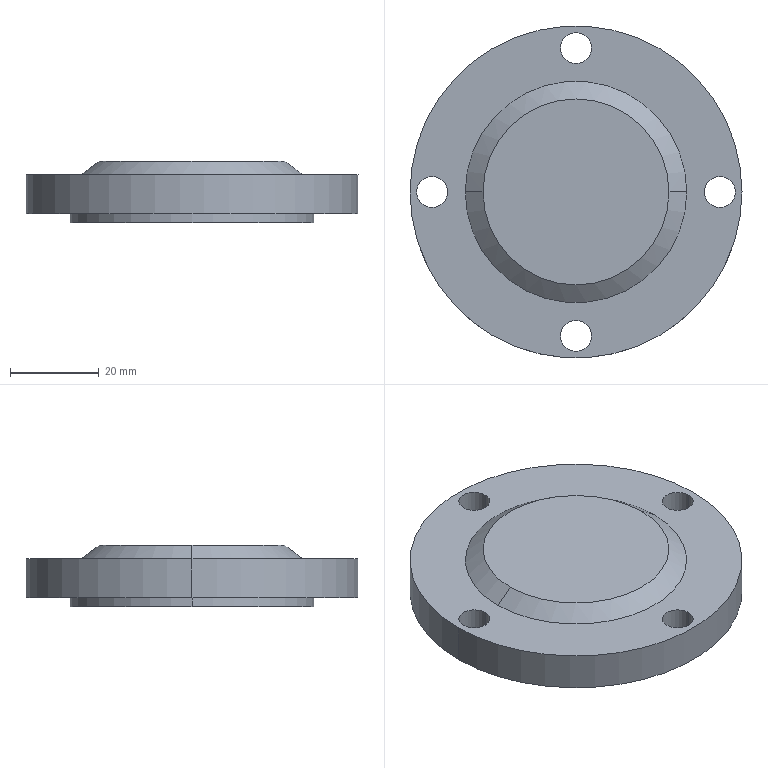Part | SolidWorks | features BaseBody 1, Chamfer 1 | 1 solid | 23 faces | box 75 x 75 x 13.8 mm | volume 30557 mm3 | cylinder 14 | plane 5 | cone 4 | commonest cylinder face diameters 7 x8 47 x2 55 x2 75 x2
STEP:
#1=CARTESIAN_POINT('',(0.,-21.5,3.4));
#2=VERTEX_POINT('',#1);
#3=CARTESIAN_POINT('',(0.,21.5,3.4));
#4=VERTEX_POINT('',#3);
#5=CARTESIAN_POINT('',(0.,0.,3.4));
#6=DIRECTION('',(0.,0.,-1.));
#7=DIRECTION('',(0.,1.,0.));
#8=AXIS2_PLACEMENT_3D('',#5,#6,#7);
#9=CIRCLE('',#8,21.5);
#10=EDGE_CURVE('',#2,#4,#9,.T.);
#11=ORIENTED_EDGE('',*,*,#10,.F.);
#12=CARTESIAN_POINT('',(0.,-23.5,1.4));
#13=VERTEX_POINT('',#12);
#14=CARTESIAN_POINT('',(0.,-21.5,3.4));
#15=DIRECTION('',(0.,-0.7071,-0.7071));
#16=VECTOR('',#15,1000.);
#17=LINE('',#14,#16);
#18=EDGE_CURVE('',#2,#13,#17,.T.);
#19=ORIENTED_EDGE('',*,*,#18,.T.);
#20=CARTESIAN_POINT('',(-23.5,0.,1.4));
#21=VERTEX_POINT('',#20);
#22=CARTESIAN_POINT('',(0.,0.,1.4));
#23=DIRECTION('',(0.,0.,1.));
#24=DIRECTION('',(0.,1.,0.));
#25=AXIS2_PLACEMENT_3D('',#22,#23,#24);
#26=CIRCLE('',#25,23.5);
#27=EDGE_CURVE('',#21,#13,#26,.T.);
#28=ORIENTED_EDGE('',*,*,#27,.F.);
#29=CARTESIAN_POINT('',(0.,23.5,1.4));
#30=VERTEX_POINT('',#29);
#31=CARTESIAN_POINT('',(0.,0.,1.4));
#32=DIRECTION('',(0.,0.,1.));
#33=DIRECTION('',(0.,1.,0.));
#34=AXIS2_PLACEMENT_3D('',#31,#32,#33);
#35=CIRCLE('',#34,23.5);
#36=EDGE_CURVE('',#30,#21,#35,.T.);
#37=ORIENTED_EDGE('',*,*,#36,.F.);
#38=CARTESIAN_POINT('',(0.,21.5,3.4));
#39=DIRECTION('',(0.,0.7071,-0.7071));
#40=VECTOR('',#39,1000.);
#41=LINE('',#38,#40);
#42=EDGE_CURVE('',#4,#30,#41,.T.);
#43=ORIENTED_EDGE('',*,*,#42,.F.);
#44=EDGE_LOOP('',(#11,#19,#28,#37,#43));
#45=FACE_OUTER_BOUND('',#44,.T.);
#46=CARTESIAN_POINT('',(0.,0.,3.4));
#47=DIRECTION('',(0.,0.,-1.));
#48=DIRECTION('',(0.,1.,0.));
#49=AXIS2_PLACEMENT_3D('',#46,#47,#48);
#50=CONICAL_SURFACE('',#49,21.5,0.7854);
#51=ADVANCED_FACE('',(#45),#50,.F.);
#52=CARTESIAN_POINT('',(-36.,0.,-4.4));
#53=VERTEX_POINT('',#52);
#54=CARTESIAN_POINT('',(-29.,0.,-4.4));
#55=VERTEX_POINT('',#54);
#56=CARTESIAN_POINT('',(-32.5,0.,-4.4));
#57=DIRECTION('',(0.,0.,1.));
#58=DIRECTION('',(1.,0.,0.));
#59=AXIS2_PLACEMENT_3D('',#56,#57,#58);
#60=CIRCLE('',#59,3.5);
#61=EDGE_CURVE('',#53,#55,#60,.T.);
#62=ORIENTED_EDGE('',*,*,#61,.F.);
#63=CARTESIAN_POINT('',(-36.,0.,4.4));
#64=VERTEX_POINT('',#63);
#65=CARTESIAN_POINT('',(-36.,0.,-5.6));
#66=DIRECTION('',(0.,0.,1.));
#67=VECTOR('',#66,1000.);
#68=LINE('',#65,#67);
#69=EDGE_CURVE('',#53,#64,#68,.T.);
#70=ORIENTED_EDGE('',*,*,#69,.T.);
#71=CARTESIAN_POINT('',(-29.,0.,4.4));
#72=VERTEX_POINT('',#71);
#73=CARTESIAN_POINT('',(-32.5,0.,4.4));
#74=DIRECTION('',(0.,0.,1.));
#75=DIRECTION('',(1.,0.,0.));
#76=AXIS2_PLACEMENT_3D('',#73,#74,#75);
#77=CIRCLE('',#76,3.5);
#78=EDGE_CURVE('',#64,#72,#77,.T.);
#79=ORIENTED_EDGE('',*,*,#78,.T.);
#80=CARTESIAN_POINT('',(-29.,0.,-5.6));
#81=DIRECTION('',(0.,0.,1.));
#82=VECTOR('',#81,1000.);
#83=LINE('',#80,#82);
#84=EDGE_CURVE('',#55,#72,#83,.T.);
#85=ORIENTED_EDGE('',*,*,#84,.F.);
#86=EDGE_LOOP('',(#62,#70,#79,#85));
#87=FACE_OUTER_BOUND('',#86,.T.);
#88=CARTESIAN_POINT('',(-32.5,0.,-5.6));
#89=DIRECTION('',(0.,0.,1.));
#90=DIRECTION('',(1.,0.,0.));
#91=AXIS2_PLACEMENT_3D('',#88,#89,#90);
#92=CYLINDRICAL_SURFACE('',#91,3.5);
#93=ADVANCED_FACE('',(#87),#92,.F.);
#94=CARTESIAN_POINT('',(-3.5,-32.5,-4.4));
#95=VERTEX_POINT('',#94);
#96=CARTESIAN_POINT('',(3.5,-32.5,-4.4));
#97=VERTEX_POINT('',#96);
#98=CARTESIAN_POINT('',(0.,-32.5,-4.4));
#99=DIRECTION('',(0.,0.,1.));
#100=DIRECTION('',(1.,0.,0.));
#101=AXIS2_PLACEMENT_3D('',#98,#99,#100);
#102=CIRCLE('',#101,3.5);
#103=EDGE_CURVE('',#95,#97,#102,.T.);
#104=ORIENTED_EDGE('',*,*,#103,.F.);
#105=CARTESIAN_POINT('',(-3.5,-32.5,4.4));
#106=VERTEX_POINT('',#105);
#107=CARTESIAN_POINT('',(-3.5,-32.5,-5.6));
#108=DIRECTION('',(0.,0.,1.));
#109=VECTOR('',#108,1000.);
#110=LINE('',#107,#109);
#111=EDGE_CURVE('',#95,#106,#110,.T.);
#112=ORIENTED_EDGE('',*,*,#111,.T.);
#113=CARTESIAN_POINT('',(3.5,-32.5,4.4));
#114=VERTEX_POINT('',#113);
#115=CARTESIAN_POINT('',(0.,-32.5,4.4));
#116=DIRECTION('',(0.,0.,1.));
#117=DIRECTION('',(1.,0.,0.));
#118=AXIS2_PLACEMENT_3D('',#115,#116,#117);
#119=CIRCLE('',#118,3.5);
#120=EDGE_CURVE('',#106,#114,#119,.T.);
#121=ORIENTED_EDGE('',*,*,#120,.T.);
#122=CARTESIAN_POINT('',(3.5,-32.5,-5.6));
#123=DIRECTION('',(0.,0.,1.));
#124=VECTOR('',#123,1000.);
#125=LINE('',#122,#124);
#126=EDGE_CURVE('',#97,#114,#125,.T.);
#127=ORIENTED_EDGE('',*,*,#126,.F.);
#128=EDGE_LOOP('',(#104,#112,#121,#127));
#129=FACE_OUTER_BOUND('',#128,.T.);
#130=CARTESIAN_POINT('',(0.,-32.5,-5.6));
#131=DIRECTION('',(0.,0.,1.));
#132=DIRECTION('',(1.,0.,0.));
#133=AXIS2_PLACEMENT_3D('',#130,#131,#132);
#134=CYLINDRICAL_SURFACE('',#133,3.5);
#135=ADVANCED_FACE('',(#129),#134,.F.);
#136=CARTESIAN_POINT('',(29.,0.,-4.4));
#137=VERTEX_POINT('',#136);
#138=CARTESIAN_POINT('',(36.,0.,-4.4));
#139=VERTEX_POINT('',#138);
#140=CARTESIAN_POINT('',(32.5,0.,-4.4));
#141=DIRECTION('',(0.,0.,1.));
#142=DIRECTION('',(1.,0.,0.));
#143=AXIS2_PLACEMENT_3D('',#140,#141,#142);
#144=CIRCLE('',#143,3.5);
#145=EDGE_CURVE('',#137,#139,#144,.T.);
#146=ORIENTED_EDGE('',*,*,#145,.F.);
#147=CARTESIAN_POINT('',(29.,0.,4.4));
#148=VERTEX_POINT('',#147);
#149=CARTESIAN_POINT('',(29.,0.,-5.6));
#150=DIRECTION('',(0.,0.,1.));
#151=VECTOR('',#150,1000.);
#152=LINE('',#149,#151);
#153=EDGE_CURVE('',#137,#148,#152,.T.);
#154=ORIENTED_EDGE('',*,*,#153,.T.);
#155=CARTESIAN_POINT('',(36.,0.,4.4));
#156=VERTEX_POINT('',#155);
#157=CARTESIAN_POINT('',(32.5,0.,4.4));
#158=DIRECTION('',(0.,0.,1.));
#159=DIRECTION('',(1.,0.,0.));
#160=AXIS2_PLACEMENT_3D('',#157,#158,#159);
#161=CIRCLE('',#160,3.5);
#162=EDGE_CURVE('',#148,#156,#161,.T.);
#163=ORIENTED_EDGE('',*,*,#162,.T.);
#164=CARTESIAN_POINT('',(36.,0.,-5.6));
#165=DIRECTION('',(0.,0.,1.));
#166=VECTOR('',#165,1000.);
#167=LINE('',#164,#166);
#168=EDGE_CURVE('',#139,#156,#167,.T.);
#169=ORIENTED_EDGE('',*,*,#168,.F.);
#170=EDGE_LOOP('',(#146,#154,#163,#169));
#171=FACE_OUTER_BOUND('',#170,.T.);
#172=CARTESIAN_POINT('',(32.5,0.,-5.6));
#173=DIRECTION('',(0.,0.,1.));
#174=DIRECTION('',(1.,0.,0.));
#175=AXIS2_PLACEMENT_3D('',#172,#173,#174);
#176=CYLINDRICAL_SURFACE('',#175,3.5);
#177=ADVANCED_FACE('',(#171),#176,.F.);
#178=CARTESIAN_POINT('',(-3.5,32.5,-4.4));
#179=VERTEX_POINT('',#178);
#180=CARTESIAN_POINT('',(3.5,32.5,-4.4));
#181=VERTEX_POINT('',#180);
#182=CARTESIAN_POINT('',(0.,32.5,-4.4));
#183=DIRECTION('',(0.,0.,1.));
#184=DIRECTION('',(1.,0.,0.));
#185=AXIS2_PLACEMENT_3D('',#182,#183,#184);
#186=CIRCLE('',#185,3.5);
#187=EDGE_CURVE('',#179,#181,#186,.T.);
#188=ORIENTED_EDGE('',*,*,#187,.F.);
#189=CARTESIAN_POINT('',(-3.5,32.5,4.4));
#190=VERTEX_POINT('',#189);
#191=CARTESIAN_POINT('',(-3.5,32.5,-5.6));
#192=DIRECTION('',(0.,0.,1.));
#193=VECTOR('',#192,1000.);
#194=LINE('',#191,#193);
#195=EDGE_CURVE('',#179,#190,#194,.T.);
#196=ORIENTED_EDGE('',*,*,#195,.T.);
#197=CARTESIAN_POINT('',(3.5,32.5,4.4));
#198=VERTEX_POINT('',#197);
#199=CARTESIAN_POINT('',(0.,32.5,4.4));
#200=DIRECTION('',(0.,0.,1.));
#201=DIRECTION('',(1.,0.,0.));
#202=AXIS2_PLACEMENT_3D('',#199,#200,#201);
#203=CIRCLE('',#202,3.5);
#204=EDGE_CURVE('',#190,#198,#203,.T.);
#205=ORIENTED_EDGE('',*,*,#204,.T.);
#206=CARTESIAN_POINT('',(3.5,32.5,-5.6));
#207=DIRECTION('',(0.,0.,1.));
#208=VECTOR('',#207,1000.);
#209=LINE('',#206,#208);
#210=EDGE_CURVE('',#181,#198,#209,.T.);
#211=ORIENTED_EDGE('',*,*,#210,.F.);
#212=EDGE_LOOP('',(#188,#196,#205,#211));
#213=FACE_OUTER_BOUND('',#212,.T.);
#214=CARTESIAN_POINT('',(0.,32.5,-5.6));
#215=DIRECTION('',(0.,0.,1.));
#216=DIRECTION('',(1.,0.,0.));
#217=AXIS2_PLACEMENT_3D('',#214,#215,#216);
#218=CYLINDRICAL_SURFACE('',#217,3.5);
#219=ADVANCED_FACE('',(#213),#218,.F.);
#220=ORIENTED_EDGE('',*,*,#27,.T.);
#221=CARTESIAN_POINT('',(23.5,0.,1.4));
#222=VERTEX_POINT('',#221);
#223=CARTESIAN_POINT('',(0.,0.,1.4));
#224=DIRECTION('',(0.,0.,1.));
#225=DIRECTION('',(0.,1.,0.));
#226=AXIS2_PLACEMENT_3D('',#223,#224,#225);
#227=CIRCLE('',#226,23.5);
#228=EDGE_CURVE('',#13,#222,#227,.T.);
#229=ORIENTED_EDGE('',*,*,#228,.T.);
#230=CARTESIAN_POINT('',(23.5,0.,-6.4));
#231=VERTEX_POINT('',#230);
#232=CARTESIAN_POINT('',(23.5,0.,3.4));
#233=DIRECTION('',(0.,0.,-1.));
#234=VECTOR('',#233,1000.);
#235=LINE('',#232,#234);
#236=EDGE_CURVE('',#222,#231,#235,.T.);
#237=ORIENTED_EDGE('',*,*,#236,.T.);
#238=CARTESIAN_POINT('',(-23.5,0.,-6.4));
#239=VERTEX_POINT('',#238);
#240=CARTESIAN_POINT('',(0.,0.,-6.4));
#241=DIRECTION('',(0.,0.,-1.));
#242=DIRECTION('',(-1.,0.,0.));
#243=AXIS2_PLACEMENT_3D('',#240,#241,#242);
#244=CIRCLE('',#243,23.5);
#245=EDGE_CURVE('',#231,#239,#244,.T.);
#246=ORIENTED_EDGE('',*,*,#245,.T.);
#247=CARTESIAN_POINT('',(-23.5,0.,3.4));
#248=DIRECTION('',(0.,0.,-1.));
#249=VECTOR('',#248,1000.);
#250=LINE('',#247,#249);
#251=EDGE_CURVE('',#21,#239,#250,.T.);
#252=ORIENTED_EDGE('',*,*,#251,.F.);
#253=EDGE_LOOP('',(#220,#229,#237,#246,#252));
#254=FACE_OUTER_BOUND('',#253,.T.);
#255=CARTESIAN_POINT('',(0.,0.,3.4));
#256=DIRECTION('',(0.,0.,-1.));
#257=DIRECTION('',(-1.,0.,0.));
#258=AXIS2_PLACEMENT_3D('',#255,#256,#257);
#259=CYLINDRICAL_SURFACE('',#258,23.5);
#260=ADVANCED_FACE('',(#254),#259,.F.);
#261=CARTESIAN_POINT('',(27.5,0.,-6.4));
#262=VERTEX_POINT('',#261);
#263=CARTESIAN_POINT('',(-27.5,0.,-6.4));
#264=VERTEX_POINT('',#263);
#265=CARTESIAN_POINT('',(0.,0.,-6.4));
#266=DIRECTION('',(0.,0.,1.));
#267=DIRECTION('',(1.,0.,0.));
#268=AXIS2_PLACEMENT_3D('',#265,#266,#267);
#269=CIRCLE('',#268,27.5);
#270=EDGE_CURVE('',#262,#264,#269,.T.);
#271=ORIENTED_EDGE('',*,*,#270,.T.);
#272=CARTESIAN_POINT('',(-27.5,0.,-4.4));
#273=VERTEX_POINT('',#272);
#274=CARTESIAN_POINT('',(-27.5,0.,-6.6));
#275=DIRECTION('',(0.,0.,1.));
#276=VECTOR('',#275,1000.);
#277=LINE('',#274,#276);
#278=EDGE_CURVE('',#264,#273,#277,.T.);
#279=ORIENTED_EDGE('',*,*,#278,.T.);
#280=CARTESIAN_POINT('',(27.5,0.,-4.4));
#281=VERTEX_POINT('',#280);
#282=CARTESIAN_POINT('',(0.,0.,-4.4));
#283=DIRECTION('',(0.,0.,-1.));
#284=DIRECTION('',(1.,0.,0.));
#285=AXIS2_PLACEMENT_3D('',#282,#283,#284);
#286=CIRCLE('',#285,27.5);
#287=EDGE_CURVE('',#273,#281,#286,.T.);
#288=ORIENTED_EDGE('',*,*,#287,.T.);
#289=CARTESIAN_POINT('',(27.5,0.,-6.6));
#290=DIRECTION('',(0.,0.,1.));
#291=VECTOR('',#290,1000.);
#292=LINE('',#289,#291);
#293=EDGE_CURVE('',#262,#281,#292,.T.);
#294=ORIENTED_EDGE('',*,*,#293,.F.);
#295=EDGE_LOOP('',(#271,#279,#288,#294));
#296=FACE_OUTER_BOUND('',#295,.T.);
#297=CARTESIAN_POINT('',(0.,0.,-6.6));
#298=DIRECTION('',(0.,0.,1.));
#299=DIRECTION('',(1.,0.,0.));
#300=AXIS2_PLACEMENT_3D('',#297,#298,#299);
#301=CYLINDRICAL_SURFACE('',#300,27.5);
#302=ADVANCED_FACE('',(#296),#301,.T.);
#303=CARTESIAN_POINT('',(-21.,0.,7.4));
#304=VERTEX_POINT('',#303);
#305=CARTESIAN_POINT('',(21.,0.,7.4));
#306=VERTEX_POINT('',#305);
#307=CARTESIAN_POINT('',(0.,0.,7.4));
#308=DIRECTION('',(0.,0.,-1.));
#309=DIRECTION('',(-1.,0.,0.));
#310=AXIS2_PLACEMENT_3D('',#307,#308,#309);
#311=CIRCLE('',#310,21.);
#312=EDGE_CURVE('',#304,#306,#311,.T.);
#313=ORIENTED_EDGE('',*,*,#312,.T.);
#314=CARTESIAN_POINT('',(25.,0.,4.4));
#315=VERTEX_POINT('',#314);
#316=CARTESIAN_POINT('',(21.,0.,7.4));
#317=DIRECTION('',(0.8,0.,-0.6));
#318=VECTOR('',#317,1000.);
#319=LINE('',#316,#318);
#320=EDGE_CURVE('',#306,#315,#319,.T.);
#321=ORIENTED_EDGE('',*,*,#320,.T.);
#322=CARTESIAN_POINT('',(-25.,0.,4.4));
#323=VERTEX_POINT('',#322);
#324=CARTESIAN_POINT('',(0.,0.,4.4));
#325=DIRECTION('',(0.,0.,-1.));
#326=DIRECTION('',(-1.,0.,0.));
#327=AXIS2_PLACEMENT_3D('',#324,#325,#326);
#328=CIRCLE('',#327,25.);
#329=EDGE_CURVE('',#323,#315,#328,.T.);
#330=ORIENTED_EDGE('',*,*,#329,.F.);
#331=CARTESIAN_POINT('',(-21.,0.,7.4));
#332=DIRECTION('',(-0.8,0.,-0.6));
#333=VECTOR('',#332,1000.);
#334=LINE('',#331,#333);
#335=EDGE_CURVE('',#304,#323,#334,.T.);
#336=ORIENTED_EDGE('',*,*,#335,.F.);
#337=EDGE_LOOP('',(#313,#321,#330,#336));
#338=FACE_OUTER_BOUND('',#337,.T.);
#339=CARTESIAN_POINT('',(0.,0.,7.4));
#340=DIRECTION('',(0.,0.,-1.));
#341=DIRECTION('',(-1.,0.,0.));
#342=AXIS2_PLACEMENT_3D('',#339,#340,#341);
#343=CONICAL_SURFACE('',#342,21.,0.9273);
#344=ADVANCED_FACE('',(#338),#343,.T.);
#345=CARTESIAN_POINT('',(37.5,0.,4.4));
#346=VERTEX_POINT('',#345);
#347=CARTESIAN_POINT('',(-37.5,0.,4.4));
#348=VERTEX_POINT('',#347);
#349=CARTESIAN_POINT('',(0.,0.,4.4));
#350=DIRECTION('',(0.,0.,1.));
#351=DIRECTION('',(1.,0.,0.));
#352=AXIS2_PLACEMENT_3D('',#349,#350,#351);
#353=CIRCLE('',#352,37.5);
#354=EDGE_CURVE('',#346,#348,#353,.T.);
#355=ORIENTED_EDGE('',*,*,#354,.F.);
#356=CARTESIAN_POINT('',(37.5,0.,-4.4));
#357=VERTEX_POINT('',#356);
#358=CARTESIAN_POINT('',(37.5,0.,4.4));
#359=DIRECTION('',(0.,0.,-1.));
#360=VECTOR('',#359,1000.);
#361=LINE('',#358,#360);
#362=EDGE_CURVE('',#346,#357,#361,.T.);
#363=ORIENTED_EDGE('',*,*,#362,.T.);
#364=CARTESIAN_POINT('',(-37.5,0.,-4.4));
#365=VERTEX_POINT('',#364);
#366=CARTESIAN_POINT('',(0.,0.,-4.4));
#367=DIRECTION('',(0.,0.,1.));
#368=DIRECTION('',(1.,0.,0.));
#369=AXIS2_PLACEMENT_3D('',#366,#367,#368);
#370=CIRCLE('',#369,37.5);
#371=EDGE_CURVE('',#357,#365,#370,.T.);
#372=ORIENTED_EDGE('',*,*,#371,.T.);
#373=CARTESIAN_POINT('',(-37.5,0.,4.4));
#374=DIRECTION('',(0.,0.,-1.));
#375=VECTOR('',#374,1000.);
#376=LINE('',#373,#375);
#377=EDGE_CURVE('',#348,#365,#376,.T.);
#378=ORIENTED_EDGE('',*,*,#377,.F.);
#379=EDGE_LOOP('',(#355,#363,#372,#378));
#380=FACE_OUTER_BOUND('',#379,.T.);
#381=CARTESIAN_POINT('',(0.,0.,4.4));
#382=DIRECTION('',(0.,0.,-1.));
#383=DIRECTION('',(-1.,0.,0.));
#384=AXIS2_PLACEMENT_3D('',#381,#382,#383);
#385=CYLINDRICAL_SURFACE('',#384,37.5);
#386=ADVANCED_FACE('',(#380),#385,.T.);
#387=CARTESIAN_POINT('',(0.,0.,3.4));
#388=DIRECTION('',(0.,0.,-1.));
#389=DIRECTION('',(0.,1.,0.));
#390=AXIS2_PLACEMENT_3D('',#387,#388,#389);
#391=CIRCLE('',#390,21.5);
#392=EDGE_CURVE('',#4,#2,#391,.T.);
#393=ORIENTED_EDGE('',*,*,#392,.T.);
#394=ORIENTED_EDGE('',*,*,#10,.T.);
#395=EDGE_LOOP('',(#393,#394));
#396=FACE_OUTER_BOUND('',#395,.T.);
#397=CARTESIAN_POINT('',(0.,0.,3.4));
#398=DIRECTION('',(0.,0.,-1.));
#399=DIRECTION('',(-1.,0.,0.));
#400=AXIS2_PLACEMENT_3D('',#397,#398,#399);
#401=PLANE('',#400);
#402=ADVANCED_FACE('',(#396),#401,.T.);
#403=ORIENTED_EDGE('',*,*,#312,.F.);
#404=CARTESIAN_POINT('',(0.,0.,7.4));
#405=DIRECTION('',(0.,0.,-1.));
#406=DIRECTION('',(-1.,0.,0.));
#407=AXIS2_PLACEMENT_3D('',#404,#405,#406);
#408=CIRCLE('',#407,21.);
#409=EDGE_CURVE('',#306,#304,#408,.T.);
#410=ORIENTED_EDGE('',*,*,#409,.F.);
#411=EDGE_LOOP('',(#403,#410));
#412=FACE_OUTER_BOUND('',#411,.T.);
#413=CARTESIAN_POINT('',(0.,0.,7.4));
#414=DIRECTION('',(0.,0.,-1.));
#415=DIRECTION('',(-1.,0.,0.));
#416=AXIS2_PLACEMENT_3D('',#413,#414,#415);
#417=PLANE('',#416);
#418=ADVANCED_FACE('',(#412),#417,.F.);
#419=CARTESIAN_POINT('',(0.,0.,-4.4));
#420=DIRECTION('',(0.,0.,-1.));
#421=DIRECTION('',(1.,0.,0.));
#422=AXIS2_PLACEMENT_3D('',#419,#420,#421);
#423=CIRCLE('',#422,27.5);
#424=EDGE_CURVE('',#281,#273,#423,.T.);
#425=ORIENTED_EDGE('',*,*,#424,.F.);
#426=ORIENTED_EDGE('',*,*,#287,.F.);
#427=EDGE_LOOP('',(#425,#426));
#428=FACE_BOUND('',#427,.T.);
#429=CARTESIAN_POINT('',(0.,32.5,-4.4));
#430=DIRECTION('',(0.,0.,1.));
#431=DIRECTION('',(1.,0.,0.));
#432=AXIS2_PLACEMENT_3D('',#429,#430,#431);
#433=CIRCLE('',#432,3.5);
#434=EDGE_CURVE('',#181,#179,#433,.T.);
#435=ORIENTED_EDGE('',*,*,#434,.T.);
#436=ORIENTED_EDGE('',*,*,#187,.T.);
#437=EDGE_LOOP('',(#435,#436));
#438=FACE_BOUND('',#437,.T.);
#439=CARTESIAN_POINT('',(32.5,0.,-4.4));
#440=DIRECTION('',(0.,0.,1.));
#441=DIRECTION('',(1.,0.,0.));
#442=AXIS2_PLACEMENT_3D('',#439,#440,#441);
#443=CIRCLE('',#442,3.5);
#444=EDGE_CURVE('',#139,#137,#443,.T.);
#445=ORIENTED_EDGE('',*,*,#444,.T.);
#446=ORIENTED_EDGE('',*,*,#145,.T.);
#447=EDGE_LOOP('',(#445,#446));
#448=FACE_BOUND('',#447,.T.);
#449=CARTESIAN_POINT('',(0.,-32.5,-4.4));
#450=DIRECTION('',(0.,0.,1.));
#451=DIRECTION('',(1.,0.,0.));
#452=AXIS2_PLACEMENT_3D('',#449,#450,#451);
#453=CIRCLE('',#452,3.5);
#454=EDGE_CURVE('',#97,#95,#453,.T.);
#455=ORIENTED_EDGE('',*,*,#454,.T.);
#456=ORIENTED_EDGE('',*,*,#103,.T.);
#457=EDGE_LOOP('',(#455,#456));
#458=FACE_BOUND('',#457,.T.);
#459=CARTESIAN_POINT('',(-32.5,0.,-4.4));
#460=DIRECTION('',(0.,0.,1.));
#461=DIRECTION('',(1.,0.,0.));
#462=AXIS2_PLACEMENT_3D('',#459,#460,#461);
#463=CIRCLE('',#462,3.5);
#464=EDGE_CURVE('',#55,#53,#463,.T.);
#465=ORIENTED_EDGE('',*,*,#464,.T.);
#466=ORIENTED_EDGE('',*,*,#61,.T.);
#467=EDGE_LOOP('',(#465,#466));
#468=FACE_BOUND('',#467,.T.);
#469=CARTESIAN_POINT('',(0.,0.,-4.4));
#470=DIRECTION('',(0.,0.,1.));
#471=DIRECTION('',(1.,0.,0.));
#472=AXIS2_PLACEMENT_3D('',#469,#470,#471);
#473=CIRCLE('',#472,37.5);
#474=EDGE_CURVE('',#365,#357,#473,.T.);
#475=ORIENTED_EDGE('',*,*,#474,.F.);
#476=ORIENTED_EDGE('',*,*,#371,.F.);
#477=EDGE_LOOP('',(#475,#476));
#478=FACE_OUTER_BOUND('',#477,.T.);
#479=CARTESIAN_POINT('',(0.,0.,-4.4));
#480=DIRECTION('',(0.,0.,1.));
#481=DIRECTION('',(0.,-1.,0.));
#482=AXIS2_PLACEMENT_3D('',#479,#480,#481);
#483=PLANE('',#482);
#484=ADVANCED_FACE('',(#428,#438,#448,#458,#468,#478),#483,.F.);
#485=ORIENTED_EDGE('',*,*,#329,.T.);
#486=CARTESIAN_POINT('',(0.,0.,4.4));
#487=DIRECTION('',(0.,0.,-1.));
#488=DIRECTION('',(-1.,0.,0.));
#489=AXIS2_PLACEMENT_3D('',#486,#487,#488);
#490=CIRCLE('',#489,25.);
#491=EDGE_CURVE('',#315,#323,#490,.T.);
#492=ORIENTED_EDGE('',*,*,#491,.T.);
#493=EDGE_LOOP('',(#485,#492));
#494=FACE_BOUND('',#493,.T.);
#495=CARTESIAN_POINT('',(0.,32.5,4.4));
#496=DIRECTION('',(0.,0.,1.));
#497=DIRECTION('',(1.,0.,0.));
#498=AXIS2_PLACEMENT_3D('',#495,#496,#497);
#499=CIRCLE('',#498,3.5);
#500=EDGE_CURVE('',#198,#190,#499,.T.);
#501=ORIENTED_EDGE('',*,*,#500,.F.);
#502=ORIENTED_EDGE('',*,*,#204,.F.);
#503=EDGE_LOOP('',(#501,#502));
#504=FACE_BOUND('',#503,.T.);
#505=CARTESIAN_POINT('',(32.5,0.,4.4));
#506=DIRECTION('',(0.,0.,1.));
#507=DIRECTION('',(1.,0.,0.));
#508=AXIS2_PLACEMENT_3D('',#505,#506,#507);
#509=CIRCLE('',#508,3.5);
#510=EDGE_CURVE('',#156,#148,#509,.T.);
#511=ORIENTED_EDGE('',*,*,#510,.F.);
#512=ORIENTED_EDGE('',*,*,#162,.F.);
#513=EDGE_LOOP('',(#511,#512));
#514=FACE_BOUND('',#513,.T.);
#515=CARTESIAN_POINT('',(0.,-32.5,4.4));
#516=DIRECTION('',(0.,0.,1.));
#517=DIRECTION('',(1.,0.,0.));
#518=AXIS2_PLACEMENT_3D('',#515,#516,#517);
#519=CIRCLE('',#518,3.5);
#520=EDGE_CURVE('',#114,#106,#519,.T.);
#521=ORIENTED_EDGE('',*,*,#520,.F.);
#522=ORIENTED_EDGE('',*,*,#120,.F.);
#523=EDGE_LOOP('',(#521,#522));
#524=FACE_BOUND('',#523,.T.);
#525=CARTESIAN_POINT('',(-32.5,0.,4.4));
#526=DIRECTION('',(0.,0.,1.));
#527=DIRECTION('',(1.,0.,0.));
#528=AXIS2_PLACEMENT_3D('',#525,#526,#527);
#529=CIRCLE('',#528,3.5);
#530=EDGE_CURVE('',#72,#64,#529,.T.);
#531=ORIENTED_EDGE('',*,*,#530,.F.);
#532=ORIENTED_EDGE('',*,*,#78,.F.);
#533=EDGE_LOOP('',(#531,#532));
#534=FACE_BOUND('',#533,.T.);
#535=CARTESIAN_POINT('',(0.,0.,4.4));
#536=DIRECTION('',(0.,0.,1.));
#537=DIRECTION('',(1.,0.,0.));
#538=AXIS2_PLACEMENT_3D('',#535,#536,#537);
#539=CIRCLE('',#538,37.5);
#540=EDGE_CURVE('',#348,#346,#539,.T.);
#541=ORIENTED_EDGE('',*,*,#540,.T.);
#542=ORIENTED_EDGE('',*,*,#354,.T.);
#543=EDGE_LOOP('',(#541,#542));
#544=FACE_OUTER_BOUND('',#543,.T.);
#545=CARTESIAN_POINT('',(0.,0.,4.4));
#546=DIRECTION('',(0.,0.,1.));
#547=DIRECTION('',(0.,-1.,0.));
#548=AXIS2_PLACEMENT_3D('',#545,#546,#547);
#549=PLANE('',#548);
#550=ADVANCED_FACE('',(#494,#504,#514,#524,#534,#544),#549,.T.);
#551=ORIENTED_EDGE('',*,*,#362,.F.);
#552=ORIENTED_EDGE('',*,*,#540,.F.);
#553=ORIENTED_EDGE('',*,*,#377,.T.);
#554=ORIENTED_EDGE('',*,*,#474,.T.);
#555=EDGE_LOOP('',(#551,#552,#553,#554));
#556=FACE_OUTER_BOUND('',#555,.T.);
#557=CARTESIAN_POINT('',(0.,0.,4.4));
#558=DIRECTION('',(0.,0.,-1.));
#559=DIRECTION('',(-1.,0.,0.));
#560=AXIS2_PLACEMENT_3D('',#557,#558,#559);
#561=CYLINDRICAL_SURFACE('',#560,37.5);
#562=ADVANCED_FACE('',(#556),#561,.T.);
#563=ORIENTED_EDGE('',*,*,#320,.F.);
#564=ORIENTED_EDGE('',*,*,#409,.T.);
#565=ORIENTED_EDGE('',*,*,#335,.T.);
#566=ORIENTED_EDGE('',*,*,#491,.F.);
#567=EDGE_LOOP('',(#563,#564,#565,#566));
#568=FACE_OUTER_BOUND('',#567,.T.);
#569=CARTESIAN_POINT('',(0.,0.,7.4));
#570=DIRECTION('',(0.,0.,-1.));
#571=DIRECTION('',(-1.,0.,0.));
#572=AXIS2_PLACEMENT_3D('',#569,#570,#571);
#573=CONICAL_SURFACE('',#572,21.,0.9273);
#574=ADVANCED_FACE('',(#568),#573,.T.);
#575=ORIENTED_EDGE('',*,*,#278,.F.);
#576=CARTESIAN_POINT('',(0.,0.,-6.4));
#577=DIRECTION('',(0.,0.,1.));
#578=DIRECTION('',(1.,0.,0.));
#579=AXIS2_PLACEMENT_3D('',#576,#577,#578);
#580=CIRCLE('',#579,27.5);
#581=EDGE_CURVE('',#264,#262,#580,.T.);
#582=ORIENTED_EDGE('',*,*,#581,.T.);
#583=ORIENTED_EDGE('',*,*,#293,.T.);
#584=ORIENTED_EDGE('',*,*,#424,.T.);
#585=EDGE_LOOP('',(#575,#582,#583,#584));
#586=FACE_OUTER_BOUND('',#585,.T.);
#587=CARTESIAN_POINT('',(0.,0.,-6.6));
#588=DIRECTION('',(0.,0.,1.));
#589=DIRECTION('',(1.,0.,0.));
#590=AXIS2_PLACEMENT_3D('',#587,#588,#589);
#591=CYLINDRICAL_SURFACE('',#590,27.5);
#592=ADVANCED_FACE('',(#586),#591,.T.);
#593=ORIENTED_EDGE('',*,*,#236,.F.);
#594=CARTESIAN_POINT('',(0.,0.,1.4));
#595=DIRECTION('',(0.,0.,1.));
#596=DIRECTION('',(0.,1.,0.));
#597=AXIS2_PLACEMENT_3D('',#594,#595,#596);
#598=CIRCLE('',#597,23.5);
#599=EDGE_CURVE('',#222,#30,#598,.T.);
#600=ORIENTED_EDGE('',*,*,#599,.T.);
#601=ORIENTED_EDGE('',*,*,#36,.T.);
#602=ORIENTED_EDGE('',*,*,#251,.T.);
#603=CARTESIAN_POINT('',(0.,0.,-6.4));
#604=DIRECTION('',(0.,0.,-1.));
#605=DIRECTION('',(-1.,0.,0.));
#606=AXIS2_PLACEMENT_3D('',#603,#604,#605);
#607=CIRCLE('',#606,23.5);
#608=EDGE_CURVE('',#239,#231,#607,.T.);
#609=ORIENTED_EDGE('',*,*,#608,.T.);
#610=EDGE_LOOP('',(#593,#600,#601,#602,#609));
#611=FACE_OUTER_BOUND('',#610,.T.);
#612=CARTESIAN_POINT('',(0.,0.,3.4));
#613=DIRECTION('',(0.,0.,-1.));
#614=DIRECTION('',(-1.,0.,0.));
#615=AXIS2_PLACEMENT_3D('',#612,#613,#614);
#616=CYLINDRICAL_SURFACE('',#615,23.5);
#617=ADVANCED_FACE('',(#611),#616,.F.);
#618=ORIENTED_EDGE('',*,*,#195,.F.);
#619=ORIENTED_EDGE('',*,*,#434,.F.);
#620=ORIENTED_EDGE('',*,*,#210,.T.);
#621=ORIENTED_EDGE('',*,*,#500,.T.);
#622=EDGE_LOOP('',(#618,#619,#620,#621));
#623=FACE_OUTER_BOUND('',#622,.T.);
#624=CARTESIAN_POINT('',(0.,32.5,-5.6));
#625=DIRECTION('',(0.,0.,1.));
#626=DIRECTION('',(1.,0.,0.));
#627=AXIS2_PLACEMENT_3D('',#624,#625,#626);
#628=CYLINDRICAL_SURFACE('',#627,3.5);
#629=ADVANCED_FACE('',(#623),#628,.F.);
#630=ORIENTED_EDGE('',*,*,#153,.F.);
#631=ORIENTED_EDGE('',*,*,#444,.F.);
#632=ORIENTED_EDGE('',*,*,#168,.T.);
#633=ORIENTED_EDGE('',*,*,#510,.T.);
#634=EDGE_LOOP('',(#630,#631,#632,#633));
#635=FACE_OUTER_BOUND('',#634,.T.);
#636=CARTESIAN_POINT('',(32.5,0.,-5.6));
#637=DIRECTION('',(0.,0.,1.));
#638=DIRECTION('',(1.,0.,0.));
#639=AXIS2_PLACEMENT_3D('',#636,#637,#638);
#640=CYLINDRICAL_SURFACE('',#639,3.5);
#641=ADVANCED_FACE('',(#635),#640,.F.);
#642=ORIENTED_EDGE('',*,*,#111,.F.);
#643=ORIENTED_EDGE('',*,*,#454,.F.);
#644=ORIENTED_EDGE('',*,*,#126,.T.);
#645=ORIENTED_EDGE('',*,*,#520,.T.);
#646=EDGE_LOOP('',(#642,#643,#644,#645));
#647=FACE_OUTER_BOUND('',#646,.T.);
#648=CARTESIAN_POINT('',(0.,-32.5,-5.6));
#649=DIRECTION('',(0.,0.,1.));
#650=DIRECTION('',(1.,0.,0.));
#651=AXIS2_PLACEMENT_3D('',#648,#649,#650);
#652=CYLINDRICAL_SURFACE('',#651,3.5);
#653=ADVANCED_FACE('',(#647),#652,.F.);
#654=ORIENTED_EDGE('',*,*,#69,.F.);
#655=ORIENTED_EDGE('',*,*,#464,.F.);
#656=ORIENTED_EDGE('',*,*,#84,.T.);
#657=ORIENTED_EDGE('',*,*,#530,.T.);
#658=EDGE_LOOP('',(#654,#655,#656,#657));
#659=FACE_OUTER_BOUND('',#658,.T.);
#660=CARTESIAN_POINT('',(-32.5,0.,-5.6));
#661=DIRECTION('',(0.,0.,1.));
#662=DIRECTION('',(1.,0.,0.));
#663=AXIS2_PLACEMENT_3D('',#660,#661,#662);
#664=CYLINDRICAL_SURFACE('',#663,3.5);
#665=ADVANCED_FACE('',(#659),#664,.F.);
#666=ORIENTED_EDGE('',*,*,#608,.F.);
#667=ORIENTED_EDGE('',*,*,#245,.F.);
#668=EDGE_LOOP('',(#666,#667));
#669=FACE_BOUND('',#668,.T.);
#670=ORIENTED_EDGE('',*,*,#270,.F.);
#671=ORIENTED_EDGE('',*,*,#581,.F.);
#672=EDGE_LOOP('',(#670,#671));
#673=FACE_OUTER_BOUND('',#672,.T.);
#674=CARTESIAN_POINT('',(0.,0.,-6.4));
#675=DIRECTION('',(0.,0.,-1.));
#676=DIRECTION('',(-1.,0.,0.));
#677=AXIS2_PLACEMENT_3D('',#674,#675,#676);
#678=PLANE('',#677);
#679=ADVANCED_FACE('',(#669,#673),#678,.T.);
#680=ORIENTED_EDGE('',*,*,#18,.F.);
#681=ORIENTED_EDGE('',*,*,#392,.F.);
#682=ORIENTED_EDGE('',*,*,#42,.T.);
#683=ORIENTED_EDGE('',*,*,#599,.F.);
#684=ORIENTED_EDGE('',*,*,#228,.F.);
#685=EDGE_LOOP('',(#680,#681,#682,#683,#684));
#686=FACE_OUTER_BOUND('',#685,.T.);
#687=CARTESIAN_POINT('',(0.,0.,3.4));
#688=DIRECTION('',(0.,0.,-1.));
#689=DIRECTION('',(0.,1.,0.));
#690=AXIS2_PLACEMENT_3D('',#687,#688,#689);
#691=CONICAL_SURFACE('',#690,21.5,0.7854);
#692=ADVANCED_FACE('',(#686),#691,.F.);
#693=CLOSED_SHELL('',(#51,#93,#135,#177,#219,#260,#302,#344,#386,#402,#418,#484,#550,#562,#574,#592,#617,#629,#641,#653,#665,#679,#692));
#694=MANIFOLD_SOLID_BREP('',#693);
#695=CARTESIAN_POINT('',(0.,0.,0.));
#696=DIRECTION('',(0.,0.,1.));
#697=DIRECTION('',(1.,0.,0.));
#698=AXIS2_PLACEMENT_3D('',#695,#696,#697);
#699=(LENGTH_UNIT()NAMED_UNIT(*)SI_UNIT(.MILLI.,.METRE.));
#700=UNCERTAINTY_MEASURE_WITH_UNIT(LENGTH_MEASURE(0.00001),#699,'','');
#701=(NAMED_UNIT(*)PLANE_ANGLE_UNIT()SI_UNIT($,.RADIAN.));
#702=(NAMED_UNIT(*)SI_UNIT($,.STERADIAN.)SOLID_ANGLE_UNIT());
#703=(GEOMETRIC_REPRESENTATION_CONTEXT(3)GLOBAL_UNCERTAINTY_ASSIGNED_CONTEXT((#700))GLOBAL_UNIT_ASSIGNED_CONTEXT((#699,#701,#702))REPRESENTATION_CONTEXT('',''));
#704=ADVANCED_BREP_SHAPE_REPRESENTATION('',(#694,#698),#703);